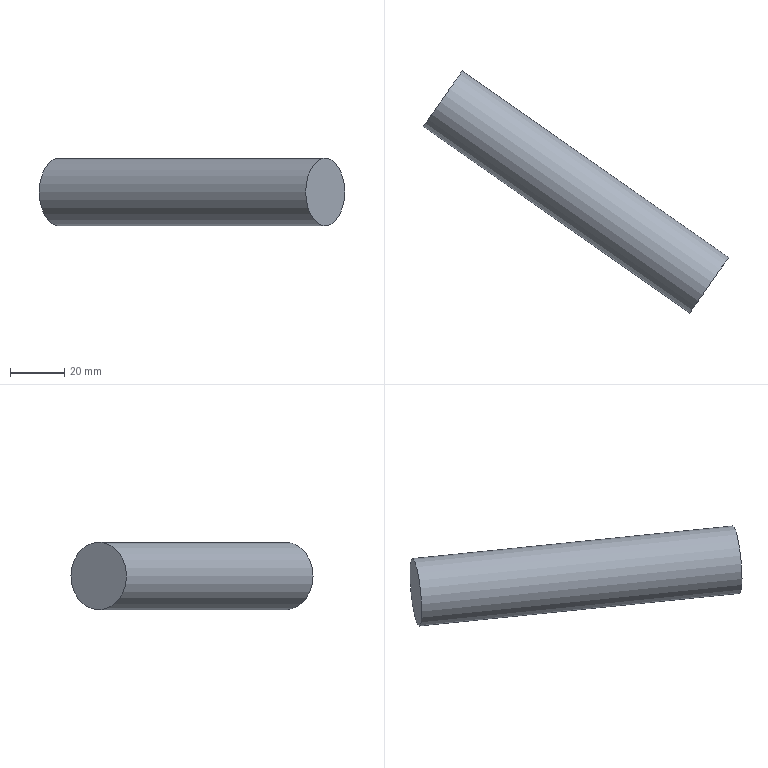Part | NX | features solid 2 | 1 solid | 3 faces | box 112.638 x 89.308 x 25 mm | volume 58905 mm3 | plane 2 | cylinder 1 | commonest cylinder face diameters 25 x1
STEP:
#1=CARTESIAN_POINT('',(-7.295,221.796,-329.036));
#2=VERTEX_POINT('',#1);
#3=CARTESIAN_POINT('',(-14.465,211.556,-329.036));
#4=DIRECTION('',(0.8192,-0.5736,0.));
#5=DIRECTION('',(0.5736,0.8192,0.));
#6=AXIS2_PLACEMENT_3D('',#3,#4,#5);
#7=CIRCLE('',#6,12.5);
#8=EDGE_CURVE('',#2,#2,#7,.T.);
#9=ORIENTED_EDGE('',*,*,#8,.F.);
#10=EDGE_LOOP('',(#9));
#11=FACE_BOUND('',#10,.T.);
#12=CARTESIAN_POINT('',(-105.593,290.625,-329.036));
#13=VERTEX_POINT('',#12);
#14=CARTESIAN_POINT('',(-112.763,280.385,-329.036));
#15=DIRECTION('',(0.8192,-0.5736,0.));
#16=DIRECTION('',(0.5736,0.8192,0.));
#17=AXIS2_PLACEMENT_3D('',#14,#15,#16);
#18=CIRCLE('',#17,12.5);
#19=EDGE_CURVE('',#13,#13,#18,.T.);
#20=ORIENTED_EDGE('',*,*,#19,.T.);
#21=EDGE_LOOP('',(#20));
#22=FACE_BOUND('',#21,.T.);
#23=CARTESIAN_POINT('',(-14.465,211.556,-329.036));
#24=DIRECTION('',(-0.8192,0.5736,0.));
#25=DIRECTION('',(-0.5736,-0.8192,0.));
#26=AXIS2_PLACEMENT_3D('',#23,#24,#25);
#27=CYLINDRICAL_SURFACE('',#26,12.5);
#28=ADVANCED_FACE('',(#11,#22),#27,.T.);
#29=ORIENTED_EDGE('',*,*,#8,.T.);
#30=EDGE_LOOP('',(#29));
#31=FACE_BOUND('',#30,.T.);
#32=CARTESIAN_POINT('',(-14.465,211.556,-329.036));
#33=DIRECTION('',(0.8192,-0.5736,0.));
#34=DIRECTION('',(0.5736,0.8192,0.));
#35=AXIS2_PLACEMENT_3D('',#32,#33,#34);
#36=PLANE('',#35);
#37=ADVANCED_FACE('',(#31),#36,.T.);
#38=ORIENTED_EDGE('',*,*,#19,.F.);
#39=EDGE_LOOP('',(#38));
#40=FACE_BOUND('',#39,.T.);
#41=CARTESIAN_POINT('',(-112.763,280.385,-329.036));
#42=DIRECTION('',(0.8192,-0.5736,0.));
#43=DIRECTION('',(0.5736,0.8192,0.));
#44=AXIS2_PLACEMENT_3D('',#41,#42,#43);
#45=PLANE('',#44);
#46=ADVANCED_FACE('',(#40),#45,.F.);
#47=CLOSED_SHELL('',(#28,#37,#46));
#48=MANIFOLD_SOLID_BREP('',#47);
#49=(LENGTH_UNIT()NAMED_UNIT(*)SI_UNIT(.MILLI.,.METRE.));
#50=UNCERTAINTY_MEASURE_WITH_UNIT(LENGTH_MEASURE(0.00001),#49,'','');
#51=(NAMED_UNIT(*)PLANE_ANGLE_UNIT()SI_UNIT($,.RADIAN.));
#52=(NAMED_UNIT(*)SI_UNIT($,.STERADIAN.)SOLID_ANGLE_UNIT());
#53=(GEOMETRIC_REPRESENTATION_CONTEXT(3)GLOBAL_UNCERTAINTY_ASSIGNED_CONTEXT((#50))GLOBAL_UNIT_ASSIGNED_CONTEXT((#49,#51,#52))REPRESENTATION_CONTEXT('',''));
#54=ADVANCED_BREP_SHAPE_REPRESENTATION('',(#48),#53);